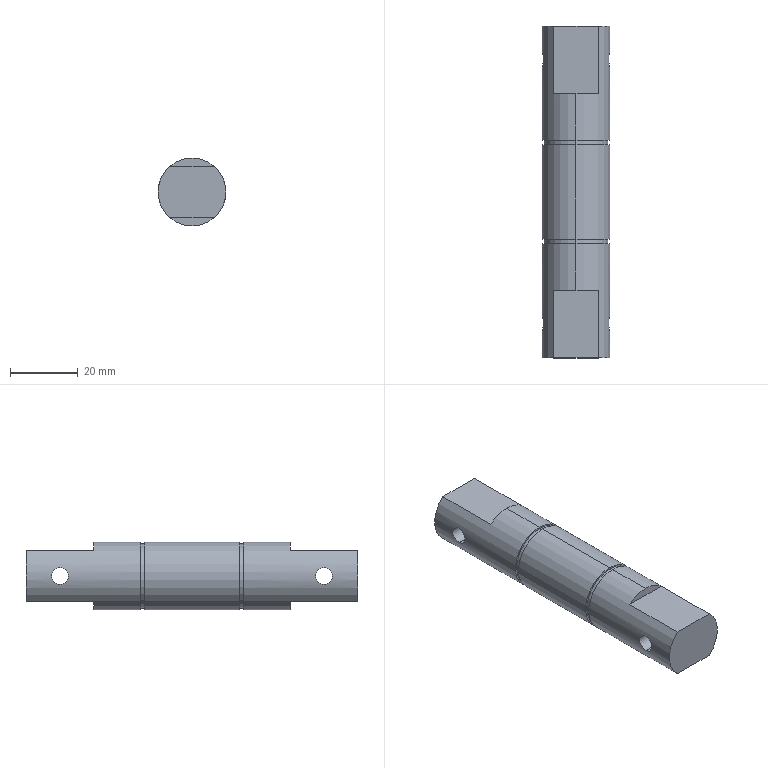Part | SolidWorks | features Extrusion 1, HoleWzd 1, ICE 1, RevCut 1 | 1 solid | 28 faces | box 20 x 98 x 20 mm | volume 28115 mm3 | cylinder 14 | plane 14 | commonest cylinder face diameters 20 x6 5 x4 19 x4
STEP:
#1=CARTESIAN_POINT('',(9.682,10.,-2.5));
#2=VERTEX_POINT('',#1);
#3=CARTESIAN_POINT('',(9.682,10.,2.5));
#4=VERTEX_POINT('',#3);
#5=CARTESIAN_POINT('',(9.682,10.,-2.5));
#6=CARTESIAN_POINT('',(9.682,9.834,-2.5));
#7=CARTESIAN_POINT('',(9.687,9.671,-2.484));
#8=CARTESIAN_POINT('',(9.703,9.351,-2.42));
#9=CARTESIAN_POINT('',(9.715,9.192,-2.371));
#10=CARTESIAN_POINT('',(9.745,8.889,-2.246));
#11=CARTESIAN_POINT('',(9.762,8.746,-2.169));
#12=CARTESIAN_POINT('',(9.801,8.475,-1.987));
#13=CARTESIAN_POINT('',(9.822,8.347,-1.882));
#14=CARTESIAN_POINT('',(9.884,8.002,-1.538));
#15=CARTESIAN_POINT('',(9.925,7.816,-1.26));
#16=CARTESIAN_POINT('',(9.968,7.629,-0.8089));
#17=CARTESIAN_POINT('',(9.98,7.581,-0.6506));
#18=CARTESIAN_POINT('',(9.996,7.516,-0.3275));
#19=CARTESIAN_POINT('',(10.,7.5,-0.1648));
#20=CARTESIAN_POINT('',(10.,7.5,0.1628));
#21=CARTESIAN_POINT('',(9.996,7.516,0.3292));
#22=CARTESIAN_POINT('',(9.98,7.581,0.6504));
#23=CARTESIAN_POINT('',(9.969,7.628,0.8066));
#24=CARTESIAN_POINT('',(9.925,7.817,1.262));
#25=CARTESIAN_POINT('',(9.884,8.001,1.537));
#26=CARTESIAN_POINT('',(9.822,8.349,1.884));
#27=CARTESIAN_POINT('',(9.801,8.474,1.987));
#28=CARTESIAN_POINT('',(9.763,8.744,2.168));
#29=CARTESIAN_POINT('',(9.745,8.891,2.246));
#30=CARTESIAN_POINT('',(9.715,9.193,2.372));
#31=CARTESIAN_POINT('',(9.703,9.348,2.419));
#32=CARTESIAN_POINT('',(9.687,9.67,2.484));
#33=CARTESIAN_POINT('',(9.682,9.836,2.5));
#34=CARTESIAN_POINT('',(9.682,10.,2.5));
#35=B_SPLINE_CURVE_WITH_KNOTS('',3,(#5,#6,#7,#8,#9,#10,#11,#12,#13,#14,#15,#16,#17,#18,#19,#20,#21,#22,#23,#24,#25,#26,#27,#28,#29,#30,#31,#32,#33,#34),.UNSPECIFIED.,.F.,.F.,(4,2,2,2,2,2,2,2,2,2,2,2,2,2,4),(0.,0.0004905,0.0009809,0.001471,0.001962,0.002943,0.003433,0.003924,0.004414,0.004905,0.005885,0.006376,0.006866,0.007357,0.007847),.UNSPECIFIED.);
#36=EDGE_CURVE('',#2,#4,#35,.T.);
#37=ORIENTED_EDGE('',*,*,#36,.T.);
#38=CARTESIAN_POINT('',(9.682,10.,2.5));
#39=CARTESIAN_POINT('',(9.682,10.327,2.5));
#40=CARTESIAN_POINT('',(9.7,10.657,2.434));
#41=CARTESIAN_POINT('',(9.745,11.109,2.247));
#42=CARTESIAN_POINT('',(9.763,11.255,2.168));
#43=CARTESIAN_POINT('',(9.801,11.526,1.987));
#44=CARTESIAN_POINT('',(9.822,11.652,1.884));
#45=CARTESIAN_POINT('',(9.863,11.882,1.653));
#46=CARTESIAN_POINT('',(9.884,11.987,1.526));
#47=CARTESIAN_POINT('',(9.922,12.168,1.255));
#48=CARTESIAN_POINT('',(9.939,12.245,1.112));
#49=CARTESIAN_POINT('',(9.968,12.372,0.808));
#50=CARTESIAN_POINT('',(9.98,12.419,0.6507));
#51=CARTESIAN_POINT('',(9.996,12.483,0.3307));
#52=CARTESIAN_POINT('',(10.,12.5,0.1656));
#53=CARTESIAN_POINT('',(10.,12.5,-0.1641));
#54=CARTESIAN_POINT('',(9.996,12.484,-0.3268));
#55=CARTESIAN_POINT('',(9.98,12.42,-0.6479));
#56=CARTESIAN_POINT('',(9.968,12.372,-0.8075));
#57=CARTESIAN_POINT('',(9.939,12.246,-1.109));
#58=CARTESIAN_POINT('',(9.922,12.17,-1.253));
#59=CARTESIAN_POINT('',(9.884,11.988,-1.525));
#60=CARTESIAN_POINT('',(9.863,11.883,-1.652));
#61=CARTESIAN_POINT('',(9.822,11.654,-1.882));
#62=CARTESIAN_POINT('',(9.801,11.527,-1.986));
#63=CARTESIAN_POINT('',(9.763,11.255,-2.168));
#64=CARTESIAN_POINT('',(9.745,11.112,-2.245));
#65=CARTESIAN_POINT('',(9.715,10.811,-2.371));
#66=CARTESIAN_POINT('',(9.703,10.651,-2.419));
#67=CARTESIAN_POINT('',(9.687,10.329,-2.484));
#68=CARTESIAN_POINT('',(9.682,10.166,-2.5));
#69=CARTESIAN_POINT('',(9.682,10.,-2.5));
#70=B_SPLINE_CURVE_WITH_KNOTS('',3,(#38,#39,#40,#41,#42,#43,#44,#45,#46,#47,#48,#49,#50,#51,#52,#53,#54,#55,#56,#57,#58,#59,#60,#61,#62,#63,#64,#65,#66,#67,#68,#69),.UNSPECIFIED.,.F.,.F.,(4,2,2,2,2,2,2,2,2,2,2,2,2,2,2,4),(0.007847,0.008828,0.009318,0.009809,0.0103,0.01079,0.01128,0.01177,0.01226,0.01275,0.01324,0.01373,0.01422,0.01471,0.0152,0.01569),.UNSPECIFIED.);
#71=EDGE_CURVE('',#4,#2,#70,.T.);
#72=ORIENTED_EDGE('',*,*,#71,.T.);
#73=EDGE_LOOP('',(#37,#72));
#74=FACE_BOUND('',#73,.T.);
#75=CARTESIAN_POINT('',(0.,33.7,10.));
#76=VERTEX_POINT('',#75);
#77=CARTESIAN_POINT('',(0.,33.7,-10.));
#78=VERTEX_POINT('',#77);
#79=CARTESIAN_POINT('',(0.,33.7,0.));
#80=DIRECTION('',(0.,1.,0.));
#81=DIRECTION('',(0.,0.,1.));
#82=AXIS2_PLACEMENT_3D('',#79,#80,#81);
#83=CIRCLE('',#82,10.);
#84=EDGE_CURVE('',#76,#78,#83,.T.);
#85=ORIENTED_EDGE('',*,*,#84,.F.);
#86=CARTESIAN_POINT('',(0.,20.,10.));
#87=VERTEX_POINT('',#86);
#88=CARTESIAN_POINT('',(0.,98.,10.));
#89=DIRECTION('',(0.,-1.,0.));
#90=VECTOR('',#89,1000.);
#91=LINE('',#88,#90);
#92=EDGE_CURVE('',#76,#87,#91,.T.);
#93=ORIENTED_EDGE('',*,*,#92,.T.);
#94=CARTESIAN_POINT('',(6.614,20.,7.5));
#95=VERTEX_POINT('',#94);
#96=CARTESIAN_POINT('',(0.,20.,0.));
#97=DIRECTION('',(0.,-1.,0.));
#98=DIRECTION('',(0.,0.,-1.));
#99=AXIS2_PLACEMENT_3D('',#96,#97,#98);
#100=CIRCLE('',#99,10.);
#101=EDGE_CURVE('',#95,#87,#100,.T.);
#102=ORIENTED_EDGE('',*,*,#101,.F.);
#103=CARTESIAN_POINT('',(6.614,0.,7.5));
#104=VERTEX_POINT('',#103);
#105=CARTESIAN_POINT('',(6.614,98.,7.5));
#106=DIRECTION('',(0.,1.,0.));
#107=VECTOR('',#106,1000.);
#108=LINE('',#105,#107);
#109=EDGE_CURVE('',#104,#95,#108,.T.);
#110=ORIENTED_EDGE('',*,*,#109,.F.);
#111=CARTESIAN_POINT('',(6.614,0.,-7.5));
#112=VERTEX_POINT('',#111);
#113=CARTESIAN_POINT('',(0.,0.,0.));
#114=DIRECTION('',(0.,1.,0.));
#115=DIRECTION('',(0.,0.,1.));
#116=AXIS2_PLACEMENT_3D('',#113,#114,#115);
#117=CIRCLE('',#116,10.);
#118=EDGE_CURVE('',#104,#112,#117,.T.);
#119=ORIENTED_EDGE('',*,*,#118,.T.);
#120=CARTESIAN_POINT('',(6.614,20.,-7.5));
#121=VERTEX_POINT('',#120);
#122=CARTESIAN_POINT('',(6.614,98.,-7.5));
#123=DIRECTION('',(0.,-1.,0.));
#124=VECTOR('',#123,1000.);
#125=LINE('',#122,#124);
#126=EDGE_CURVE('',#121,#112,#125,.T.);
#127=ORIENTED_EDGE('',*,*,#126,.F.);
#128=CARTESIAN_POINT('',(0.,20.,-10.));
#129=VERTEX_POINT('',#128);
#130=CARTESIAN_POINT('',(0.,20.,0.));
#131=DIRECTION('',(0.,-1.,0.));
#132=DIRECTION('',(0.,0.,-1.));
#133=AXIS2_PLACEMENT_3D('',#130,#131,#132);
#134=CIRCLE('',#133,10.);
#135=EDGE_CURVE('',#129,#121,#134,.T.);
#136=ORIENTED_EDGE('',*,*,#135,.F.);
#137=CARTESIAN_POINT('',(0.,98.,-10.));
#138=DIRECTION('',(0.,-1.,0.));
#139=VECTOR('',#138,1000.);
#140=LINE('',#137,#139);
#141=EDGE_CURVE('',#78,#129,#140,.T.);
#142=ORIENTED_EDGE('',*,*,#141,.F.);
#143=EDGE_LOOP('',(#85,#93,#102,#110,#119,#127,#136,#142));
#144=FACE_OUTER_BOUND('',#143,.T.);
#145=CARTESIAN_POINT('',(0.,98.,0.));
#146=DIRECTION('',(0.,-1.,0.));
#147=DIRECTION('',(0.,0.,-1.));
#148=AXIS2_PLACEMENT_3D('',#145,#146,#147);
#149=CYLINDRICAL_SURFACE('',#148,10.);
#150=ADVANCED_FACE('',(#74,#144),#149,.T.);
#151=CARTESIAN_POINT('',(-9.682,10.,2.5));
#152=VERTEX_POINT('',#151);
#153=CARTESIAN_POINT('',(-9.682,10.,-2.5));
#154=VERTEX_POINT('',#153);
#155=CARTESIAN_POINT('',(-9.682,10.,2.5));
#156=CARTESIAN_POINT('',(-9.682,9.835,2.5));
#157=CARTESIAN_POINT('',(-9.687,9.672,2.484));
#158=CARTESIAN_POINT('',(-9.703,9.351,2.42));
#159=CARTESIAN_POINT('',(-9.715,9.192,2.371));
#160=CARTESIAN_POINT('',(-9.745,8.89,2.246));
#161=CARTESIAN_POINT('',(-9.762,8.747,2.169));
#162=CARTESIAN_POINT('',(-9.801,8.474,1.987));
#163=CARTESIAN_POINT('',(-9.822,8.347,1.883));
#164=CARTESIAN_POINT('',(-9.863,8.118,1.653));
#165=CARTESIAN_POINT('',(-9.884,8.013,1.526));
#166=CARTESIAN_POINT('',(-9.922,7.831,1.254));
#167=CARTESIAN_POINT('',(-9.939,7.754,1.111));
#168=CARTESIAN_POINT('',(-9.968,7.629,0.8095));
#169=CARTESIAN_POINT('',(-9.98,7.58,0.6502));
#170=CARTESIAN_POINT('',(-9.996,7.516,0.3279));
#171=CARTESIAN_POINT('',(-10.,7.5,0.1644));
#172=CARTESIAN_POINT('',(-10.,7.5,-0.1673));
#173=CARTESIAN_POINT('',(-9.996,7.517,-0.3303));
#174=CARTESIAN_POINT('',(-9.98,7.581,-0.6507));
#175=CARTESIAN_POINT('',(-9.968,7.629,-0.8098));
#176=CARTESIAN_POINT('',(-9.939,7.755,-1.112));
#177=CARTESIAN_POINT('',(-9.922,7.832,-1.255));
#178=CARTESIAN_POINT('',(-9.884,8.014,-1.527));
#179=CARTESIAN_POINT('',(-9.863,8.119,-1.654));
#180=CARTESIAN_POINT('',(-9.801,8.463,-1.999));
#181=CARTESIAN_POINT('',(-9.759,8.741,-2.184));
#182=CARTESIAN_POINT('',(-9.715,9.192,-2.371));
#183=CARTESIAN_POINT('',(-9.703,9.351,-2.42));
#184=CARTESIAN_POINT('',(-9.687,9.674,-2.484));
#185=CARTESIAN_POINT('',(-9.682,9.836,-2.5));
#186=CARTESIAN_POINT('',(-9.682,10.,-2.5));
#187=B_SPLINE_CURVE_WITH_KNOTS('',3,(#155,#156,#157,#158,#159,#160,#161,#162,#163,#164,#165,#166,#167,#168,#169,#170,#171,#172,#173,#174,#175,#176,#177,#178,#179,#180,#181,#182,#183,#184,#185,#186),.UNSPECIFIED.,.F.,.F.,(4,2,2,2,2,2,2,2,2,2,2,2,2,2,2,4),(0.01177,0.01226,0.01275,0.01324,0.01373,0.01422,0.01471,0.0152,0.01569,0.01618,0.01667,0.01717,0.01766,0.01864,0.01913,0.01962),.UNSPECIFIED.);
#188=EDGE_CURVE('',#152,#154,#187,.T.);
#189=ORIENTED_EDGE('',*,*,#188,.F.);
#190=CARTESIAN_POINT('',(10.,10.,2.5));
#191=DIRECTION('',(1.,0.,0.));
#192=VECTOR('',#191,1000.);
#193=LINE('',#190,#192);
#194=EDGE_CURVE('',#152,#4,#193,.T.);
#195=ORIENTED_EDGE('',*,*,#194,.T.);
#196=ORIENTED_EDGE('',*,*,#36,.F.);
#197=CARTESIAN_POINT('',(10.,10.,-2.5));
#198=DIRECTION('',(1.,0.,0.));
#199=VECTOR('',#198,1000.);
#200=LINE('',#197,#199);
#201=EDGE_CURVE('',#154,#2,#200,.T.);
#202=ORIENTED_EDGE('',*,*,#201,.F.);
#203=EDGE_LOOP('',(#189,#195,#196,#202));
#204=FACE_OUTER_BOUND('',#203,.T.);
#205=CARTESIAN_POINT('',(10.,10.,0.));
#206=DIRECTION('',(1.,0.,0.));
#207=DIRECTION('',(0.,0.,-1.));
#208=AXIS2_PLACEMENT_3D('',#205,#206,#207);
#209=CYLINDRICAL_SURFACE('',#208,2.5);
#210=ADVANCED_FACE('',(#204),#209,.F.);
#211=CARTESIAN_POINT('',(0.,33.7,9.5));
#212=VERTEX_POINT('',#211);
#213=CARTESIAN_POINT('',(0.,33.7,-9.5));
#214=VERTEX_POINT('',#213);
#215=CARTESIAN_POINT('',(0.,33.7,0.));
#216=DIRECTION('',(0.,1.,0.));
#217=DIRECTION('',(0.,0.,1.));
#218=AXIS2_PLACEMENT_3D('',#215,#216,#217);
#219=CIRCLE('',#218,9.5);
#220=EDGE_CURVE('',#212,#214,#219,.T.);
#221=ORIENTED_EDGE('',*,*,#220,.T.);
#222=CARTESIAN_POINT('',(0.,35.,-9.5));
#223=VERTEX_POINT('',#222);
#224=CARTESIAN_POINT('',(0.,98.,-9.5));
#225=DIRECTION('',(0.,1.,0.));
#226=VECTOR('',#225,1000.);
#227=LINE('',#224,#226);
#228=EDGE_CURVE('',#214,#223,#227,.T.);
#229=ORIENTED_EDGE('',*,*,#228,.T.);
#230=CARTESIAN_POINT('',(0.,35.,9.5));
#231=VERTEX_POINT('',#230);
#232=CARTESIAN_POINT('',(0.,35.,0.));
#233=DIRECTION('',(0.,1.,0.));
#234=DIRECTION('',(0.,0.,1.));
#235=AXIS2_PLACEMENT_3D('',#232,#233,#234);
#236=CIRCLE('',#235,9.5);
#237=EDGE_CURVE('',#231,#223,#236,.T.);
#238=ORIENTED_EDGE('',*,*,#237,.F.);
#239=CARTESIAN_POINT('',(0.,98.,9.5));
#240=DIRECTION('',(0.,1.,0.));
#241=VECTOR('',#240,1000.);
#242=LINE('',#239,#241);
#243=EDGE_CURVE('',#212,#231,#242,.T.);
#244=ORIENTED_EDGE('',*,*,#243,.F.);
#245=EDGE_LOOP('',(#221,#229,#238,#244));
#246=FACE_OUTER_BOUND('',#245,.T.);
#247=CARTESIAN_POINT('',(0.,98.,0.));
#248=DIRECTION('',(0.,1.,0.));
#249=DIRECTION('',(0.,0.,1.));
#250=AXIS2_PLACEMENT_3D('',#247,#248,#249);
#251=CYLINDRICAL_SURFACE('',#250,9.5);
#252=ADVANCED_FACE('',(#246),#251,.T.);
#253=CARTESIAN_POINT('',(0.,63.,10.));
#254=VERTEX_POINT('',#253);
#255=CARTESIAN_POINT('',(0.,63.,-10.));
#256=VERTEX_POINT('',#255);
#257=CARTESIAN_POINT('',(0.,63.,0.));
#258=DIRECTION('',(0.,1.,0.));
#259=DIRECTION('',(0.,0.,1.));
#260=AXIS2_PLACEMENT_3D('',#257,#258,#259);
#261=CIRCLE('',#260,10.);
#262=EDGE_CURVE('',#254,#256,#261,.T.);
#263=ORIENTED_EDGE('',*,*,#262,.F.);
#264=CARTESIAN_POINT('',(0.,35.,10.));
#265=VERTEX_POINT('',#264);
#266=CARTESIAN_POINT('',(0.,98.,10.));
#267=DIRECTION('',(0.,-1.,0.));
#268=VECTOR('',#267,1000.);
#269=LINE('',#266,#268);
#270=EDGE_CURVE('',#254,#265,#269,.T.);
#271=ORIENTED_EDGE('',*,*,#270,.T.);
#272=CARTESIAN_POINT('',(0.,35.,-10.));
#273=VERTEX_POINT('',#272);
#274=CARTESIAN_POINT('',(0.,35.,0.));
#275=DIRECTION('',(0.,1.,0.));
#276=DIRECTION('',(0.,0.,1.));
#277=AXIS2_PLACEMENT_3D('',#274,#275,#276);
#278=CIRCLE('',#277,10.);
#279=EDGE_CURVE('',#265,#273,#278,.T.);
#280=ORIENTED_EDGE('',*,*,#279,.T.);
#281=CARTESIAN_POINT('',(0.,98.,-10.));
#282=DIRECTION('',(0.,-1.,0.));
#283=VECTOR('',#282,1000.);
#284=LINE('',#281,#283);
#285=EDGE_CURVE('',#256,#273,#284,.T.);
#286=ORIENTED_EDGE('',*,*,#285,.F.);
#287=EDGE_LOOP('',(#263,#271,#280,#286));
#288=FACE_OUTER_BOUND('',#287,.T.);
#289=CARTESIAN_POINT('',(0.,98.,0.));
#290=DIRECTION('',(0.,-1.,0.));
#291=DIRECTION('',(0.,0.,-1.));
#292=AXIS2_PLACEMENT_3D('',#289,#290,#291);
#293=CYLINDRICAL_SURFACE('',#292,10.);
#294=ADVANCED_FACE('',(#288),#293,.T.);
#295=CARTESIAN_POINT('',(0.,63.,9.5));
#296=VERTEX_POINT('',#295);
#297=CARTESIAN_POINT('',(0.,63.,-9.5));
#298=VERTEX_POINT('',#297);
#299=CARTESIAN_POINT('',(0.,63.,0.));
#300=DIRECTION('',(0.,1.,0.));
#301=DIRECTION('',(0.,0.,1.));
#302=AXIS2_PLACEMENT_3D('',#299,#300,#301);
#303=CIRCLE('',#302,9.5);
#304=EDGE_CURVE('',#296,#298,#303,.T.);
#305=ORIENTED_EDGE('',*,*,#304,.T.);
#306=CARTESIAN_POINT('',(0.,64.3,-9.5));
#307=VERTEX_POINT('',#306);
#308=CARTESIAN_POINT('',(0.,98.,-9.5));
#309=DIRECTION('',(0.,1.,0.));
#310=VECTOR('',#309,1000.);
#311=LINE('',#308,#310);
#312=EDGE_CURVE('',#298,#307,#311,.T.);
#313=ORIENTED_EDGE('',*,*,#312,.T.);
#314=CARTESIAN_POINT('',(0.,64.3,9.5));
#315=VERTEX_POINT('',#314);
#316=CARTESIAN_POINT('',(0.,64.3,0.));
#317=DIRECTION('',(0.,1.,0.));
#318=DIRECTION('',(0.,0.,1.));
#319=AXIS2_PLACEMENT_3D('',#316,#317,#318);
#320=CIRCLE('',#319,9.5);
#321=EDGE_CURVE('',#315,#307,#320,.T.);
#322=ORIENTED_EDGE('',*,*,#321,.F.);
#323=CARTESIAN_POINT('',(0.,98.,9.5));
#324=DIRECTION('',(0.,1.,0.));
#325=VECTOR('',#324,1000.);
#326=LINE('',#323,#325);
#327=EDGE_CURVE('',#296,#315,#326,.T.);
#328=ORIENTED_EDGE('',*,*,#327,.F.);
#329=EDGE_LOOP('',(#305,#313,#322,#328));
#330=FACE_OUTER_BOUND('',#329,.T.);
#331=CARTESIAN_POINT('',(0.,98.,0.));
#332=DIRECTION('',(0.,1.,0.));
#333=DIRECTION('',(0.,0.,1.));
#334=AXIS2_PLACEMENT_3D('',#331,#332,#333);
#335=CYLINDRICAL_SURFACE('',#334,9.5);
#336=ADVANCED_FACE('',(#330),#335,.T.);
#337=CARTESIAN_POINT('',(-9.682,88.,2.5));
#338=VERTEX_POINT('',#337);
#339=CARTESIAN_POINT('',(-9.682,88.,-2.5));
#340=VERTEX_POINT('',#339);
#341=CARTESIAN_POINT('',(-9.682,88.,2.5));
#342=CARTESIAN_POINT('',(-9.682,87.835,2.5));
#343=CARTESIAN_POINT('',(-9.687,87.672,2.484));
#344=CARTESIAN_POINT('',(-9.703,87.351,2.42));
#345=CARTESIAN_POINT('',(-9.715,87.192,2.371));
#346=CARTESIAN_POINT('',(-9.745,86.89,2.246));
#347=CARTESIAN_POINT('',(-9.762,86.747,2.169));
#348=CARTESIAN_POINT('',(-9.801,86.474,1.987));
#349=CARTESIAN_POINT('',(-9.822,86.347,1.883));
#350=CARTESIAN_POINT('',(-9.863,86.118,1.653));
#351=CARTESIAN_POINT('',(-9.884,86.013,1.526));
#352=CARTESIAN_POINT('',(-9.922,85.831,1.254));
#353=CARTESIAN_POINT('',(-9.939,85.754,1.111));
#354=CARTESIAN_POINT('',(-9.968,85.629,0.8095));
#355=CARTESIAN_POINT('',(-9.98,85.58,0.6502));
#356=CARTESIAN_POINT('',(-9.996,85.516,0.3279));
#357=CARTESIAN_POINT('',(-10.,85.5,0.1644));
#358=CARTESIAN_POINT('',(-10.,85.5,-0.1673));
#359=CARTESIAN_POINT('',(-9.996,85.517,-0.3303));
#360=CARTESIAN_POINT('',(-9.98,85.581,-0.6507));
#361=CARTESIAN_POINT('',(-9.968,85.629,-0.8098));
#362=CARTESIAN_POINT('',(-9.939,85.755,-1.112));
#363=CARTESIAN_POINT('',(-9.922,85.832,-1.255));
#364=CARTESIAN_POINT('',(-9.884,86.014,-1.527));
#365=CARTESIAN_POINT('',(-9.863,86.119,-1.654));
#366=CARTESIAN_POINT('',(-9.801,86.463,-1.999));
#367=CARTESIAN_POINT('',(-9.759,86.741,-2.184));
#368=CARTESIAN_POINT('',(-9.715,87.192,-2.371));
#369=CARTESIAN_POINT('',(-9.703,87.351,-2.42));
#370=CARTESIAN_POINT('',(-9.687,87.674,-2.484));
#371=CARTESIAN_POINT('',(-9.682,87.836,-2.5));
#372=CARTESIAN_POINT('',(-9.682,88.,-2.5));
#373=B_SPLINE_CURVE_WITH_KNOTS('',3,(#341,#342,#343,#344,#345,#346,#347,#348,#349,#350,#351,#352,#353,#354,#355,#356,#357,#358,#359,#360,#361,#362,#363,#364,#365,#366,#367,#368,#369,#370,#371,#372),.UNSPECIFIED.,.F.,.F.,(4,2,2,2,2,2,2,2,2,2,2,2,2,2,2,4),(0.01177,0.01226,0.01275,0.01324,0.01373,0.01422,0.01471,0.0152,0.01569,0.01618,0.01667,0.01717,0.01766,0.01864,0.01913,0.01962),.UNSPECIFIED.);
#374=EDGE_CURVE('',#338,#340,#373,.T.);
#375=ORIENTED_EDGE('',*,*,#374,.F.);
#376=CARTESIAN_POINT('',(9.682,88.,2.5));
#377=VERTEX_POINT('',#376);
#378=CARTESIAN_POINT('',(10.,88.,2.5));
#379=DIRECTION('',(1.,0.,0.));
#380=VECTOR('',#379,1000.);
#381=LINE('',#378,#380);
#382=EDGE_CURVE('',#338,#377,#381,.T.);
#383=ORIENTED_EDGE('',*,*,#382,.T.);
#384=CARTESIAN_POINT('',(9.682,88.,-2.5));
#385=VERTEX_POINT('',#384);
#386=CARTESIAN_POINT('',(9.682,88.,-2.5));
#387=CARTESIAN_POINT('',(9.682,87.834,-2.5));
#388=CARTESIAN_POINT('',(9.687,87.671,-2.484));
#389=CARTESIAN_POINT('',(9.703,87.351,-2.42));
#390=CARTESIAN_POINT('',(9.715,87.192,-2.371));
#391=CARTESIAN_POINT('',(9.745,86.889,-2.246));
#392=CARTESIAN_POINT('',(9.762,86.746,-2.169));
#393=CARTESIAN_POINT('',(9.801,86.475,-1.987));
#394=CARTESIAN_POINT('',(9.822,86.347,-1.882));
#395=CARTESIAN_POINT('',(9.884,86.002,-1.538));
#396=CARTESIAN_POINT('',(9.925,85.816,-1.26));
#397=CARTESIAN_POINT('',(9.968,85.629,-0.8089));
#398=CARTESIAN_POINT('',(9.98,85.581,-0.6506));
#399=CARTESIAN_POINT('',(9.996,85.516,-0.3275));
#400=CARTESIAN_POINT('',(10.,85.5,-0.1648));
#401=CARTESIAN_POINT('',(10.,85.5,0.1628));
#402=CARTESIAN_POINT('',(9.996,85.516,0.3292));
#403=CARTESIAN_POINT('',(9.98,85.581,0.6504));
#404=CARTESIAN_POINT('',(9.969,85.628,0.8066));
#405=CARTESIAN_POINT('',(9.925,85.817,1.262));
#406=CARTESIAN_POINT('',(9.884,86.001,1.537));
#407=CARTESIAN_POINT('',(9.822,86.349,1.884));
#408=CARTESIAN_POINT('',(9.801,86.474,1.987));
#409=CARTESIAN_POINT('',(9.763,86.744,2.168));
#410=CARTESIAN_POINT('',(9.745,86.891,2.246));
#411=CARTESIAN_POINT('',(9.715,87.193,2.372));
#412=CARTESIAN_POINT('',(9.703,87.348,2.419));
#413=CARTESIAN_POINT('',(9.687,87.67,2.484));
#414=CARTESIAN_POINT('',(9.682,87.836,2.5));
#415=CARTESIAN_POINT('',(9.682,88.,2.5));
#416=B_SPLINE_CURVE_WITH_KNOTS('',3,(#386,#387,#388,#389,#390,#391,#392,#393,#394,#395,#396,#397,#398,#399,#400,#401,#402,#403,#404,#405,#406,#407,#408,#409,#410,#411,#412,#413,#414,#415),.UNSPECIFIED.,.F.,.F.,(4,2,2,2,2,2,2,2,2,2,2,2,2,2,4),(0.,0.0004905,0.0009809,0.001471,0.001962,0.002943,0.003433,0.003924,0.004414,0.004905,0.005885,0.006376,0.006866,0.007357,0.007847),.UNSPECIFIED.);
#417=EDGE_CURVE('',#385,#377,#416,.T.);
#418=ORIENTED_EDGE('',*,*,#417,.F.);
#419=CARTESIAN_POINT('',(10.,88.,-2.5));
#420=DIRECTION('',(1.,0.,0.));
#421=VECTOR('',#420,1000.);
#422=LINE('',#419,#421);
#423=EDGE_CURVE('',#340,#385,#422,.T.);
#424=ORIENTED_EDGE('',*,*,#423,.F.);
#425=EDGE_LOOP('',(#375,#383,#418,#424));
#426=FACE_OUTER_BOUND('',#425,.T.);
#427=CARTESIAN_POINT('',(10.,88.,0.));
#428=DIRECTION('',(1.,0.,0.));
#429=DIRECTION('',(0.,0.,-1.));
#430=AXIS2_PLACEMENT_3D('',#427,#428,#429);
#431=CYLINDRICAL_SURFACE('',#430,2.5);
#432=ADVANCED_FACE('',(#426),#431,.F.);
#433=ORIENTED_EDGE('',*,*,#417,.T.);
#434=CARTESIAN_POINT('',(9.682,88.,2.5));
#435=CARTESIAN_POINT('',(9.682,88.327,2.5));
#436=CARTESIAN_POINT('',(9.7,88.657,2.434));
#437=CARTESIAN_POINT('',(9.745,89.109,2.247));
#438=CARTESIAN_POINT('',(9.763,89.255,2.168));
#439=CARTESIAN_POINT('',(9.801,89.526,1.987));
#440=CARTESIAN_POINT('',(9.822,89.652,1.884));
#441=CARTESIAN_POINT('',(9.863,89.882,1.653));
#442=CARTESIAN_POINT('',(9.884,89.987,1.526));
#443=CARTESIAN_POINT('',(9.922,90.168,1.255));
#444=CARTESIAN_POINT('',(9.939,90.245,1.112));
#445=CARTESIAN_POINT('',(9.968,90.372,0.808));
#446=CARTESIAN_POINT('',(9.98,90.419,0.6507));
#447=CARTESIAN_POINT('',(9.996,90.483,0.3307));
#448=CARTESIAN_POINT('',(10.,90.5,0.1656));
#449=CARTESIAN_POINT('',(10.,90.5,-0.1641));
#450=CARTESIAN_POINT('',(9.996,90.484,-0.3268));
#451=CARTESIAN_POINT('',(9.98,90.42,-0.6479));
#452=CARTESIAN_POINT('',(9.968,90.372,-0.8075));
#453=CARTESIAN_POINT('',(9.939,90.246,-1.109));
#454=CARTESIAN_POINT('',(9.922,90.17,-1.253));
#455=CARTESIAN_POINT('',(9.884,89.988,-1.525));
#456=CARTESIAN_POINT('',(9.863,89.883,-1.652));
#457=CARTESIAN_POINT('',(9.822,89.654,-1.882));
#458=CARTESIAN_POINT('',(9.801,89.527,-1.986));
#459=CARTESIAN_POINT('',(9.763,89.255,-2.168));
#460=CARTESIAN_POINT('',(9.745,89.112,-2.245));
#461=CARTESIAN_POINT('',(9.715,88.811,-2.371));
#462=CARTESIAN_POINT('',(9.703,88.651,-2.419));
#463=CARTESIAN_POINT('',(9.687,88.329,-2.484));
#464=CARTESIAN_POINT('',(9.682,88.166,-2.5));
#465=CARTESIAN_POINT('',(9.682,88.,-2.5));
#466=B_SPLINE_CURVE_WITH_KNOTS('',3,(#434,#435,#436,#437,#438,#439,#440,#441,#442,#443,#444,#445,#446,#447,#448,#449,#450,#451,#452,#453,#454,#455,#456,#457,#458,#459,#460,#461,#462,#463,#464,#465),.UNSPECIFIED.,.F.,.F.,(4,2,2,2,2,2,2,2,2,2,2,2,2,2,2,4),(0.007847,0.008828,0.009318,0.009809,0.0103,0.01079,0.01128,0.01177,0.01226,0.01275,0.01324,0.01373,0.01422,0.01471,0.0152,0.01569),.UNSPECIFIED.);
#467=EDGE_CURVE('',#377,#385,#466,.T.);
#468=ORIENTED_EDGE('',*,*,#467,.T.);
#469=EDGE_LOOP('',(#433,#468));
#470=FACE_BOUND('',#469,.T.);
#471=CARTESIAN_POINT('',(0.,78.,10.));
#472=VERTEX_POINT('',#471);
#473=CARTESIAN_POINT('',(6.614,78.,7.5));
#474=VERTEX_POINT('',#473);
#475=CARTESIAN_POINT('',(0.,78.,0.));
#476=DIRECTION('',(0.,1.,0.));
#477=DIRECTION('',(0.,0.,1.));
#478=AXIS2_PLACEMENT_3D('',#475,#476,#477);
#479=CIRCLE('',#478,10.);
#480=EDGE_CURVE('',#472,#474,#479,.T.);
#481=ORIENTED_EDGE('',*,*,#480,.F.);
#482=CARTESIAN_POINT('',(0.,64.3,10.));
#483=VERTEX_POINT('',#482);
#484=CARTESIAN_POINT('',(0.,98.,10.));
#485=DIRECTION('',(0.,-1.,0.));
#486=VECTOR('',#485,1000.);
#487=LINE('',#484,#486);
#488=EDGE_CURVE('',#472,#483,#487,.T.);
#489=ORIENTED_EDGE('',*,*,#488,.T.);
#490=CARTESIAN_POINT('',(0.,64.3,-10.));
#491=VERTEX_POINT('',#490);
#492=CARTESIAN_POINT('',(0.,64.3,0.));
#493=DIRECTION('',(0.,1.,0.));
#494=DIRECTION('',(0.,0.,1.));
#495=AXIS2_PLACEMENT_3D('',#492,#493,#494);
#496=CIRCLE('',#495,10.);
#497=EDGE_CURVE('',#483,#491,#496,.T.);
#498=ORIENTED_EDGE('',*,*,#497,.T.);
#499=CARTESIAN_POINT('',(0.,78.,-10.));
#500=VERTEX_POINT('',#499);
#501=CARTESIAN_POINT('',(0.,98.,-10.));
#502=DIRECTION('',(0.,-1.,0.));
#503=VECTOR('',#502,1000.);
#504=LINE('',#501,#503);
#505=EDGE_CURVE('',#500,#491,#504,.T.);
#506=ORIENTED_EDGE('',*,*,#505,.F.);
#507=CARTESIAN_POINT('',(6.614,78.,-7.5));
#508=VERTEX_POINT('',#507);
#509=CARTESIAN_POINT('',(0.,78.,0.));
#510=DIRECTION('',(0.,1.,0.));
#511=DIRECTION('',(0.,0.,1.));
#512=AXIS2_PLACEMENT_3D('',#509,#510,#511);
#513=CIRCLE('',#512,10.);
#514=EDGE_CURVE('',#508,#500,#513,.T.);
#515=ORIENTED_EDGE('',*,*,#514,.F.);
#516=CARTESIAN_POINT('',(6.614,98.,-7.5));
#517=VERTEX_POINT('',#516);
#518=CARTESIAN_POINT('',(6.614,98.,-7.5));
#519=DIRECTION('',(0.,-1.,0.));
#520=VECTOR('',#519,1000.);
#521=LINE('',#518,#520);
#522=EDGE_CURVE('',#517,#508,#521,.T.);
#523=ORIENTED_EDGE('',*,*,#522,.F.);
#524=CARTESIAN_POINT('',(6.614,98.,7.5));
#525=VERTEX_POINT('',#524);
#526=CARTESIAN_POINT('',(0.,98.,0.));
#527=DIRECTION('',(0.,1.,0.));
#528=DIRECTION('',(0.,0.,1.));
#529=AXIS2_PLACEMENT_3D('',#526,#527,#528);
#530=CIRCLE('',#529,10.);
#531=EDGE_CURVE('',#525,#517,#530,.T.);
#532=ORIENTED_EDGE('',*,*,#531,.F.);
#533=CARTESIAN_POINT('',(6.614,98.,7.5));
#534=DIRECTION('',(0.,1.,0.));
#535=VECTOR('',#534,1000.);
#536=LINE('',#533,#535);
#537=EDGE_CURVE('',#474,#525,#536,.T.);
#538=ORIENTED_EDGE('',*,*,#537,.F.);
#539=EDGE_LOOP('',(#481,#489,#498,#506,#515,#523,#532,#538));
#540=FACE_OUTER_BOUND('',#539,.T.);
#541=CARTESIAN_POINT('',(0.,98.,0.));
#542=DIRECTION('',(0.,-1.,0.));
#543=DIRECTION('',(0.,0.,-1.));
#544=AXIS2_PLACEMENT_3D('',#541,#542,#543);
#545=CYLINDRICAL_SURFACE('',#544,10.);
#546=ADVANCED_FACE('',(#470,#540),#545,.T.);
#547=ORIENTED_EDGE('',*,*,#488,.F.);
#548=CARTESIAN_POINT('',(-6.614,78.,7.5));
#549=VERTEX_POINT('',#548);
#550=CARTESIAN_POINT('',(0.,78.,0.));
#551=DIRECTION('',(0.,1.,0.));
#552=DIRECTION('',(0.,0.,1.));
#553=AXIS2_PLACEMENT_3D('',#550,#551,#552);
#554=CIRCLE('',#553,10.);
#555=EDGE_CURVE('',#549,#472,#554,.T.);
#556=ORIENTED_EDGE('',*,*,#555,.F.);
#557=CARTESIAN_POINT('',(-6.614,98.,7.5));
#558=VERTEX_POINT('',#557);
#559=CARTESIAN_POINT('',(-6.614,98.,7.5));
#560=DIRECTION('',(0.,-1.,0.));
#561=VECTOR('',#560,1000.);
#562=LINE('',#559,#561);
#563=EDGE_CURVE('',#558,#549,#562,.T.);
#564=ORIENTED_EDGE('',*,*,#563,.F.);
#565=CARTESIAN_POINT('',(-6.614,98.,-7.5));
#566=VERTEX_POINT('',#565);
#567=CARTESIAN_POINT('',(0.,98.,0.));
#568=DIRECTION('',(0.,1.,0.));
#569=DIRECTION('',(0.,0.,1.));
#570=AXIS2_PLACEMENT_3D('',#567,#568,#569);
#571=CIRCLE('',#570,10.);
#572=EDGE_CURVE('',#566,#558,#571,.T.);
#573=ORIENTED_EDGE('',*,*,#572,.F.);
#574=CARTESIAN_POINT('',(-6.614,78.,-7.5));
#575=VERTEX_POINT('',#574);
#576=CARTESIAN_POINT('',(-6.614,98.,-7.5));
#577=DIRECTION('',(0.,1.,0.));
#578=VECTOR('',#577,1000.);
#579=LINE('',#576,#578);
#580=EDGE_CURVE('',#575,#566,#579,.T.);
#581=ORIENTED_EDGE('',*,*,#580,.F.);
#582=CARTESIAN_POINT('',(0.,78.,0.));
#583=DIRECTION('',(0.,1.,0.));
#584=DIRECTION('',(0.,0.,1.));
#585=AXIS2_PLACEMENT_3D('',#582,#583,#584);
#586=CIRCLE('',#585,10.);
#587=EDGE_CURVE('',#500,#575,#586,.T.);
#588=ORIENTED_EDGE('',*,*,#587,.F.);
#589=ORIENTED_EDGE('',*,*,#505,.T.);
#590=CARTESIAN_POINT('',(0.,64.3,0.));
#591=DIRECTION('',(0.,1.,0.));
#592=DIRECTION('',(0.,0.,1.));
#593=AXIS2_PLACEMENT_3D('',#590,#591,#592);
#594=CIRCLE('',#593,10.);
#595=EDGE_CURVE('',#491,#483,#594,.T.);
#596=ORIENTED_EDGE('',*,*,#595,.T.);
#597=EDGE_LOOP('',(#547,#556,#564,#573,#581,#588,#589,#596));
#598=FACE_OUTER_BOUND('',#597,.T.);
#599=CARTESIAN_POINT('',(-9.682,88.,-2.5));
#600=CARTESIAN_POINT('',(-9.682,88.164,-2.5));
#601=CARTESIAN_POINT('',(-9.687,88.33,-2.484));
#602=CARTESIAN_POINT('',(-9.703,88.651,-2.419));
#603=CARTESIAN_POINT('',(-9.715,88.807,-2.372));
#604=CARTESIAN_POINT('',(-9.76,89.263,-2.183));
#605=CARTESIAN_POINT('',(-9.801,89.537,-1.999));
#606=CARTESIAN_POINT('',(-9.863,89.884,-1.651));
#607=CARTESIAN_POINT('',(-9.884,89.987,-1.526));
#608=CARTESIAN_POINT('',(-9.922,90.168,-1.255));
#609=CARTESIAN_POINT('',(-9.94,90.247,-1.109));
#610=CARTESIAN_POINT('',(-9.969,90.372,-0.807));
#611=CARTESIAN_POINT('',(-9.98,90.419,-0.6511));
#612=CARTESIAN_POINT('',(-9.996,90.484,-0.3291));
#613=CARTESIAN_POINT('',(-10.,90.5,-0.1631));
#614=CARTESIAN_POINT('',(-10.,90.5,0.3274));
#615=CARTESIAN_POINT('',(-9.983,90.434,0.6576));
#616=CARTESIAN_POINT('',(-9.939,90.246,1.109));
#617=CARTESIAN_POINT('',(-9.922,90.168,1.256));
#618=CARTESIAN_POINT('',(-9.884,89.986,1.527));
#619=CARTESIAN_POINT('',(-9.863,89.883,1.652));
#620=CARTESIAN_POINT('',(-9.822,89.653,1.883));
#621=CARTESIAN_POINT('',(-9.801,89.525,1.988));
#622=CARTESIAN_POINT('',(-9.763,89.255,2.168));
#623=CARTESIAN_POINT('',(-9.745,89.111,2.245));
#624=CARTESIAN_POINT('',(-9.715,88.807,2.372));
#625=CARTESIAN_POINT('',(-9.703,88.65,2.42));
#626=CARTESIAN_POINT('',(-9.687,88.33,2.483));
#627=CARTESIAN_POINT('',(-9.682,88.165,2.5));
#628=CARTESIAN_POINT('',(-9.682,88.,2.5));
#629=B_SPLINE_CURVE_WITH_KNOTS('',3,(#599,#600,#601,#602,#603,#604,#605,#606,#607,#608,#609,#610,#611,#612,#613,#614,#615,#616,#617,#618,#619,#620,#621,#622,#623,#624,#625,#626,#627,#628),.UNSPECIFIED.,.F.,.F.,(4,2,2,2,2,2,2,2,2,2,2,2,2,2,4),(0.003925,0.004415,0.004905,0.005886,0.006377,0.006867,0.007357,0.007848,0.008829,0.009319,0.009809,0.0103,0.01079,0.01128,0.01177),.UNSPECIFIED.);
#630=EDGE_CURVE('',#340,#338,#629,.T.);
#631=ORIENTED_EDGE('',*,*,#630,.T.);
#632=ORIENTED_EDGE('',*,*,#374,.T.);
#633=EDGE_LOOP('',(#631,#632));
#634=FACE_BOUND('',#633,.T.);
#635=CARTESIAN_POINT('',(0.,98.,0.));
#636=DIRECTION('',(0.,-1.,0.));
#637=DIRECTION('',(0.,0.,-1.));
#638=AXIS2_PLACEMENT_3D('',#635,#636,#637);
#639=CYLINDRICAL_SURFACE('',#638,10.);
#640=ADVANCED_FACE('',(#598,#634),#639,.T.);
#641=ORIENTED_EDGE('',*,*,#572,.T.);
#642=CARTESIAN_POINT('',(0.,98.,7.5));
#643=DIRECTION('',(1.,0.,0.));
#644=VECTOR('',#643,1000.);
#645=LINE('',#642,#644);
#646=EDGE_CURVE('',#558,#525,#645,.T.);
#647=ORIENTED_EDGE('',*,*,#646,.T.);
#648=ORIENTED_EDGE('',*,*,#531,.T.);
#649=CARTESIAN_POINT('',(0.,98.,-7.5));
#650=DIRECTION('',(-1.,0.,0.));
#651=VECTOR('',#650,1000.);
#652=LINE('',#649,#651);
#653=EDGE_CURVE('',#517,#566,#652,.T.);
#654=ORIENTED_EDGE('',*,*,#653,.T.);
#655=EDGE_LOOP('',(#641,#647,#648,#654));
#656=FACE_OUTER_BOUND('',#655,.T.);
#657=CARTESIAN_POINT('',(0.,98.,0.));
#658=DIRECTION('',(0.,1.,0.));
#659=DIRECTION('',(0.,0.,1.));
#660=AXIS2_PLACEMENT_3D('',#657,#658,#659);
#661=PLANE('',#660);
#662=ADVANCED_FACE('',(#656),#661,.T.);
#663=CARTESIAN_POINT('',(10.,78.,-7.5));
#664=DIRECTION('',(-1.,0.,0.));
#665=VECTOR('',#664,1000.);
#666=LINE('',#663,#665);
#667=EDGE_CURVE('',#508,#575,#666,.T.);
#668=ORIENTED_EDGE('',*,*,#667,.F.);
#669=ORIENTED_EDGE('',*,*,#514,.T.);
#670=ORIENTED_EDGE('',*,*,#587,.T.);
#671=EDGE_LOOP('',(#668,#669,#670));
#672=FACE_OUTER_BOUND('',#671,.T.);
#673=CARTESIAN_POINT('',(10.,78.,-10.));
#674=DIRECTION('',(0.,1.,0.));
#675=DIRECTION('',(0.,0.,1.));
#676=AXIS2_PLACEMENT_3D('',#673,#674,#675);
#677=PLANE('',#676);
#678=ADVANCED_FACE('',(#672),#677,.T.);
#679=ORIENTED_EDGE('',*,*,#522,.T.);
#680=ORIENTED_EDGE('',*,*,#667,.T.);
#681=ORIENTED_EDGE('',*,*,#580,.T.);
#682=ORIENTED_EDGE('',*,*,#653,.F.);
#683=EDGE_LOOP('',(#679,#680,#681,#682));
#684=FACE_OUTER_BOUND('',#683,.T.);
#685=CARTESIAN_POINT('',(10.,98.,-7.5));
#686=DIRECTION('',(0.,0.,-1.));
#687=DIRECTION('',(0.,1.,0.));
#688=AXIS2_PLACEMENT_3D('',#685,#686,#687);
#689=PLANE('',#688);
#690=ADVANCED_FACE('',(#684),#689,.T.);
#691=ORIENTED_EDGE('',*,*,#555,.T.);
#692=ORIENTED_EDGE('',*,*,#480,.T.);
#693=CARTESIAN_POINT('',(10.,78.,7.5));
#694=DIRECTION('',(-1.,0.,0.));
#695=VECTOR('',#694,1000.);
#696=LINE('',#693,#695);
#697=EDGE_CURVE('',#474,#549,#696,.T.);
#698=ORIENTED_EDGE('',*,*,#697,.T.);
#699=EDGE_LOOP('',(#691,#692,#698));
#700=FACE_OUTER_BOUND('',#699,.T.);
#701=CARTESIAN_POINT('',(10.,78.,10.));
#702=DIRECTION('',(0.,1.,0.));
#703=DIRECTION('',(0.,0.,1.));
#704=AXIS2_PLACEMENT_3D('',#701,#702,#703);
#705=PLANE('',#704);
#706=ADVANCED_FACE('',(#700),#705,.T.);
#707=ORIENTED_EDGE('',*,*,#563,.T.);
#708=ORIENTED_EDGE('',*,*,#697,.F.);
#709=ORIENTED_EDGE('',*,*,#537,.T.);
#710=ORIENTED_EDGE('',*,*,#646,.F.);
#711=EDGE_LOOP('',(#707,#708,#709,#710));
#712=FACE_OUTER_BOUND('',#711,.T.);
#713=CARTESIAN_POINT('',(10.,98.,7.5));
#714=DIRECTION('',(0.,0.,1.));
#715=DIRECTION('',(0.,-1.,0.));
#716=AXIS2_PLACEMENT_3D('',#713,#714,#715);
#717=PLANE('',#716);
#718=ADVANCED_FACE('',(#712),#717,.T.);
#719=ORIENTED_EDGE('',*,*,#382,.F.);
#720=ORIENTED_EDGE('',*,*,#630,.F.);
#721=ORIENTED_EDGE('',*,*,#423,.T.);
#722=ORIENTED_EDGE('',*,*,#467,.F.);
#723=EDGE_LOOP('',(#719,#720,#721,#722));
#724=FACE_OUTER_BOUND('',#723,.T.);
#725=CARTESIAN_POINT('',(10.,88.,0.));
#726=DIRECTION('',(1.,0.,0.));
#727=DIRECTION('',(0.,0.,-1.));
#728=AXIS2_PLACEMENT_3D('',#725,#726,#727);
#729=CYLINDRICAL_SURFACE('',#728,2.5);
#730=ADVANCED_FACE('',(#724),#729,.F.);
#731=ORIENTED_EDGE('',*,*,#304,.F.);
#732=CARTESIAN_POINT('',(0.,63.,0.));
#733=DIRECTION('',(0.,1.,0.));
#734=DIRECTION('',(0.,0.,1.));
#735=AXIS2_PLACEMENT_3D('',#732,#733,#734);
#736=CIRCLE('',#735,9.5);
#737=EDGE_CURVE('',#298,#296,#736,.T.);
#738=ORIENTED_EDGE('',*,*,#737,.F.);
#739=EDGE_LOOP('',(#731,#738));
#740=FACE_BOUND('',#739,.T.);
#741=CARTESIAN_POINT('',(0.,63.,0.));
#742=DIRECTION('',(0.,1.,0.));
#743=DIRECTION('',(0.,0.,1.));
#744=AXIS2_PLACEMENT_3D('',#741,#742,#743);
#745=CIRCLE('',#744,10.);
#746=EDGE_CURVE('',#256,#254,#745,.T.);
#747=ORIENTED_EDGE('',*,*,#746,.T.);
#748=ORIENTED_EDGE('',*,*,#262,.T.);
#749=EDGE_LOOP('',(#747,#748));
#750=FACE_OUTER_BOUND('',#749,.T.);
#751=CARTESIAN_POINT('',(-10.,63.,0.));
#752=DIRECTION('',(0.,-1.,0.));
#753=DIRECTION('',(0.,0.,-1.));
#754=AXIS2_PLACEMENT_3D('',#751,#752,#753);
#755=PLANE('',#754);
#756=ADVANCED_FACE('',(#740,#750),#755,.F.);
#757=ORIENTED_EDGE('',*,*,#312,.F.);
#758=ORIENTED_EDGE('',*,*,#737,.T.);
#759=ORIENTED_EDGE('',*,*,#327,.T.);
#760=CARTESIAN_POINT('',(0.,64.3,0.));
#761=DIRECTION('',(0.,1.,0.));
#762=DIRECTION('',(0.,0.,1.));
#763=AXIS2_PLACEMENT_3D('',#760,#761,#762);
#764=CIRCLE('',#763,9.5);
#765=EDGE_CURVE('',#307,#315,#764,.T.);
#766=ORIENTED_EDGE('',*,*,#765,.F.);
#767=EDGE_LOOP('',(#757,#758,#759,#766));
#768=FACE_OUTER_BOUND('',#767,.T.);
#769=CARTESIAN_POINT('',(0.,98.,0.));
#770=DIRECTION('',(0.,1.,0.));
#771=DIRECTION('',(0.,0.,1.));
#772=AXIS2_PLACEMENT_3D('',#769,#770,#771);
#773=CYLINDRICAL_SURFACE('',#772,9.5);
#774=ADVANCED_FACE('',(#768),#773,.T.);
#775=ORIENTED_EDGE('',*,*,#595,.F.);
#776=ORIENTED_EDGE('',*,*,#497,.F.);
#777=EDGE_LOOP('',(#775,#776));
#778=FACE_OUTER_BOUND('',#777,.T.);
#779=ORIENTED_EDGE('',*,*,#321,.T.);
#780=ORIENTED_EDGE('',*,*,#765,.T.);
#781=EDGE_LOOP('',(#779,#780));
#782=FACE_BOUND('',#781,.T.);
#783=CARTESIAN_POINT('',(-10.,64.3,0.));
#784=DIRECTION('',(0.,1.,0.));
#785=DIRECTION('',(0.,0.,1.));
#786=AXIS2_PLACEMENT_3D('',#783,#784,#785);
#787=PLANE('',#786);
#788=ADVANCED_FACE('',(#778,#782),#787,.F.);
#789=ORIENTED_EDGE('',*,*,#270,.F.);
#790=ORIENTED_EDGE('',*,*,#746,.F.);
#791=ORIENTED_EDGE('',*,*,#285,.T.);
#792=CARTESIAN_POINT('',(0.,35.,0.));
#793=DIRECTION('',(0.,1.,0.));
#794=DIRECTION('',(0.,0.,1.));
#795=AXIS2_PLACEMENT_3D('',#792,#793,#794);
#796=CIRCLE('',#795,10.);
#797=EDGE_CURVE('',#273,#265,#796,.T.);
#798=ORIENTED_EDGE('',*,*,#797,.T.);
#799=EDGE_LOOP('',(#789,#790,#791,#798));
#800=FACE_OUTER_BOUND('',#799,.T.);
#801=CARTESIAN_POINT('',(0.,98.,0.));
#802=DIRECTION('',(0.,-1.,0.));
#803=DIRECTION('',(0.,0.,-1.));
#804=AXIS2_PLACEMENT_3D('',#801,#802,#803);
#805=CYLINDRICAL_SURFACE('',#804,10.);
#806=ADVANCED_FACE('',(#800),#805,.T.);
#807=ORIENTED_EDGE('',*,*,#220,.F.);
#808=CARTESIAN_POINT('',(0.,33.7,0.));
#809=DIRECTION('',(0.,1.,0.));
#810=DIRECTION('',(0.,0.,1.));
#811=AXIS2_PLACEMENT_3D('',#808,#809,#810);
#812=CIRCLE('',#811,9.5);
#813=EDGE_CURVE('',#214,#212,#812,.T.);
#814=ORIENTED_EDGE('',*,*,#813,.F.);
#815=EDGE_LOOP('',(#807,#814));
#816=FACE_BOUND('',#815,.T.);
#817=CARTESIAN_POINT('',(0.,33.7,0.));
#818=DIRECTION('',(0.,1.,0.));
#819=DIRECTION('',(0.,0.,1.));
#820=AXIS2_PLACEMENT_3D('',#817,#818,#819);
#821=CIRCLE('',#820,10.);
#822=EDGE_CURVE('',#78,#76,#821,.T.);
#823=ORIENTED_EDGE('',*,*,#822,.T.);
#824=ORIENTED_EDGE('',*,*,#84,.T.);
#825=EDGE_LOOP('',(#823,#824));
#826=FACE_OUTER_BOUND('',#825,.T.);
#827=CARTESIAN_POINT('',(-10.,33.7,0.));
#828=DIRECTION('',(0.,-1.,0.));
#829=DIRECTION('',(0.,0.,-1.));
#830=AXIS2_PLACEMENT_3D('',#827,#828,#829);
#831=PLANE('',#830);
#832=ADVANCED_FACE('',(#816,#826),#831,.F.);
#833=ORIENTED_EDGE('',*,*,#228,.F.);
#834=ORIENTED_EDGE('',*,*,#813,.T.);
#835=ORIENTED_EDGE('',*,*,#243,.T.);
#836=CARTESIAN_POINT('',(0.,35.,0.));
#837=DIRECTION('',(0.,1.,0.));
#838=DIRECTION('',(0.,0.,1.));
#839=AXIS2_PLACEMENT_3D('',#836,#837,#838);
#840=CIRCLE('',#839,9.5);
#841=EDGE_CURVE('',#223,#231,#840,.T.);
#842=ORIENTED_EDGE('',*,*,#841,.F.);
#843=EDGE_LOOP('',(#833,#834,#835,#842));
#844=FACE_OUTER_BOUND('',#843,.T.);
#845=CARTESIAN_POINT('',(0.,98.,0.));
#846=DIRECTION('',(0.,1.,0.));
#847=DIRECTION('',(0.,0.,1.));
#848=AXIS2_PLACEMENT_3D('',#845,#846,#847);
#849=CYLINDRICAL_SURFACE('',#848,9.5);
#850=ADVANCED_FACE('',(#844),#849,.T.);
#851=ORIENTED_EDGE('',*,*,#797,.F.);
#852=ORIENTED_EDGE('',*,*,#279,.F.);
#853=EDGE_LOOP('',(#851,#852));
#854=FACE_OUTER_BOUND('',#853,.T.);
#855=ORIENTED_EDGE('',*,*,#237,.T.);
#856=ORIENTED_EDGE('',*,*,#841,.T.);
#857=EDGE_LOOP('',(#855,#856));
#858=FACE_BOUND('',#857,.T.);
#859=CARTESIAN_POINT('',(-10.,35.,0.));
#860=DIRECTION('',(0.,1.,0.));
#861=DIRECTION('',(0.,0.,1.));
#862=AXIS2_PLACEMENT_3D('',#859,#860,#861);
#863=PLANE('',#862);
#864=ADVANCED_FACE('',(#854,#858),#863,.F.);
#865=ORIENTED_EDGE('',*,*,#194,.F.);
#866=CARTESIAN_POINT('',(-9.682,10.,-2.5));
#867=CARTESIAN_POINT('',(-9.682,10.164,-2.5));
#868=CARTESIAN_POINT('',(-9.687,10.33,-2.484));
#869=CARTESIAN_POINT('',(-9.703,10.651,-2.419));
#870=CARTESIAN_POINT('',(-9.715,10.807,-2.372));
#871=CARTESIAN_POINT('',(-9.76,11.263,-2.183));
#872=CARTESIAN_POINT('',(-9.801,11.537,-1.999));
#873=CARTESIAN_POINT('',(-9.863,11.884,-1.651));
#874=CARTESIAN_POINT('',(-9.884,11.987,-1.526));
#875=CARTESIAN_POINT('',(-9.922,12.168,-1.255));
#876=CARTESIAN_POINT('',(-9.94,12.247,-1.109));
#877=CARTESIAN_POINT('',(-9.969,12.372,-0.807));
#878=CARTESIAN_POINT('',(-9.98,12.419,-0.6511));
#879=CARTESIAN_POINT('',(-9.996,12.484,-0.3291));
#880=CARTESIAN_POINT('',(-10.,12.5,-0.1631));
#881=CARTESIAN_POINT('',(-10.,12.5,0.3274));
#882=CARTESIAN_POINT('',(-9.983,12.434,0.6576));
#883=CARTESIAN_POINT('',(-9.939,12.246,1.109));
#884=CARTESIAN_POINT('',(-9.922,12.168,1.256));
#885=CARTESIAN_POINT('',(-9.884,11.986,1.527));
#886=CARTESIAN_POINT('',(-9.863,11.883,1.652));
#887=CARTESIAN_POINT('',(-9.822,11.653,1.883));
#888=CARTESIAN_POINT('',(-9.801,11.525,1.988));
#889=CARTESIAN_POINT('',(-9.763,11.255,2.168));
#890=CARTESIAN_POINT('',(-9.745,11.111,2.245));
#891=CARTESIAN_POINT('',(-9.715,10.807,2.372));
#892=CARTESIAN_POINT('',(-9.703,10.65,2.42));
#893=CARTESIAN_POINT('',(-9.687,10.33,2.483));
#894=CARTESIAN_POINT('',(-9.682,10.165,2.5));
#895=CARTESIAN_POINT('',(-9.682,10.,2.5));
#896=B_SPLINE_CURVE_WITH_KNOTS('',3,(#866,#867,#868,#869,#870,#871,#872,#873,#874,#875,#876,#877,#878,#879,#880,#881,#882,#883,#884,#885,#886,#887,#888,#889,#890,#891,#892,#893,#894,#895),.UNSPECIFIED.,.F.,.F.,(4,2,2,2,2,2,2,2,2,2,2,2,2,2,4),(0.003925,0.004415,0.004905,0.005886,0.006377,0.006867,0.007357,0.007848,0.008829,0.009319,0.009809,0.0103,0.01079,0.01128,0.01177),.UNSPECIFIED.);
#897=EDGE_CURVE('',#154,#152,#896,.T.);
#898=ORIENTED_EDGE('',*,*,#897,.F.);
#899=ORIENTED_EDGE('',*,*,#201,.T.);
#900=ORIENTED_EDGE('',*,*,#71,.F.);
#901=EDGE_LOOP('',(#865,#898,#899,#900));
#902=FACE_OUTER_BOUND('',#901,.T.);
#903=CARTESIAN_POINT('',(10.,10.,0.));
#904=DIRECTION('',(1.,0.,0.));
#905=DIRECTION('',(0.,0.,-1.));
#906=AXIS2_PLACEMENT_3D('',#903,#904,#905);
#907=CYLINDRICAL_SURFACE('',#906,2.5);
#908=ADVANCED_FACE('',(#902),#907,.F.);
#909=CARTESIAN_POINT('',(-6.614,20.,7.5));
#910=VERTEX_POINT('',#909);
#911=CARTESIAN_POINT('',(10.,20.,7.5));
#912=DIRECTION('',(-1.,0.,0.));
#913=VECTOR('',#912,1000.);
#914=LINE('',#911,#913);
#915=EDGE_CURVE('',#95,#910,#914,.T.);
#916=ORIENTED_EDGE('',*,*,#915,.F.);
#917=ORIENTED_EDGE('',*,*,#101,.T.);
#918=CARTESIAN_POINT('',(0.,20.,0.));
#919=DIRECTION('',(0.,-1.,0.));
#920=DIRECTION('',(0.,0.,-1.));
#921=AXIS2_PLACEMENT_3D('',#918,#919,#920);
#922=CIRCLE('',#921,10.);
#923=EDGE_CURVE('',#87,#910,#922,.T.);
#924=ORIENTED_EDGE('',*,*,#923,.T.);
#925=EDGE_LOOP('',(#916,#917,#924));
#926=FACE_OUTER_BOUND('',#925,.T.);
#927=CARTESIAN_POINT('',(10.,20.,10.));
#928=DIRECTION('',(0.,-1.,0.));
#929=DIRECTION('',(0.,0.,-1.));
#930=AXIS2_PLACEMENT_3D('',#927,#928,#929);
#931=PLANE('',#930);
#932=ADVANCED_FACE('',(#926),#931,.T.);
#933=CARTESIAN_POINT('',(-6.614,0.,7.5));
#934=VERTEX_POINT('',#933);
#935=CARTESIAN_POINT('',(-6.614,98.,7.5));
#936=DIRECTION('',(0.,-1.,0.));
#937=VECTOR('',#936,1000.);
#938=LINE('',#935,#937);
#939=EDGE_CURVE('',#910,#934,#938,.T.);
#940=ORIENTED_EDGE('',*,*,#939,.T.);
#941=CARTESIAN_POINT('',(0.,0.,7.5));
#942=DIRECTION('',(1.,0.,0.));
#943=VECTOR('',#942,1000.);
#944=LINE('',#941,#943);
#945=EDGE_CURVE('',#934,#104,#944,.T.);
#946=ORIENTED_EDGE('',*,*,#945,.T.);
#947=ORIENTED_EDGE('',*,*,#109,.T.);
#948=ORIENTED_EDGE('',*,*,#915,.T.);
#949=EDGE_LOOP('',(#940,#946,#947,#948));
#950=FACE_OUTER_BOUND('',#949,.T.);
#951=CARTESIAN_POINT('',(10.,0.,7.5));
#952=DIRECTION('',(0.,0.,1.));
#953=DIRECTION('',(0.,-1.,0.));
#954=AXIS2_PLACEMENT_3D('',#951,#952,#953);
#955=PLANE('',#954);
#956=ADVANCED_FACE('',(#950),#955,.T.);
#957=CARTESIAN_POINT('',(-6.614,0.,-7.5));
#958=VERTEX_POINT('',#957);
#959=CARTESIAN_POINT('',(0.,0.,-7.5));
#960=DIRECTION('',(-1.,0.,0.));
#961=VECTOR('',#960,1000.);
#962=LINE('',#959,#961);
#963=EDGE_CURVE('',#112,#958,#962,.T.);
#964=ORIENTED_EDGE('',*,*,#963,.F.);
#965=ORIENTED_EDGE('',*,*,#118,.F.);
#966=ORIENTED_EDGE('',*,*,#945,.F.);
#967=CARTESIAN_POINT('',(0.,0.,0.));
#968=DIRECTION('',(0.,1.,0.));
#969=DIRECTION('',(0.,0.,1.));
#970=AXIS2_PLACEMENT_3D('',#967,#968,#969);
#971=CIRCLE('',#970,10.);
#972=EDGE_CURVE('',#958,#934,#971,.T.);
#973=ORIENTED_EDGE('',*,*,#972,.F.);
#974=EDGE_LOOP('',(#964,#965,#966,#973));
#975=FACE_OUTER_BOUND('',#974,.T.);
#976=CARTESIAN_POINT('',(0.,0.,0.));
#977=DIRECTION('',(0.,1.,0.));
#978=DIRECTION('',(0.,0.,1.));
#979=AXIS2_PLACEMENT_3D('',#976,#977,#978);
#980=PLANE('',#979);
#981=ADVANCED_FACE('',(#975),#980,.F.);
#982=CARTESIAN_POINT('',(-6.614,20.,-7.5));
#983=VERTEX_POINT('',#982);
#984=CARTESIAN_POINT('',(0.,20.,0.));
#985=DIRECTION('',(0.,-1.,0.));
#986=DIRECTION('',(0.,0.,-1.));
#987=AXIS2_PLACEMENT_3D('',#984,#985,#986);
#988=CIRCLE('',#987,10.);
#989=EDGE_CURVE('',#983,#129,#988,.T.);
#990=ORIENTED_EDGE('',*,*,#989,.T.);
#991=ORIENTED_EDGE('',*,*,#135,.T.);
#992=CARTESIAN_POINT('',(10.,20.,-7.5));
#993=DIRECTION('',(-1.,0.,0.));
#994=VECTOR('',#993,1000.);
#995=LINE('',#992,#994);
#996=EDGE_CURVE('',#121,#983,#995,.T.);
#997=ORIENTED_EDGE('',*,*,#996,.T.);
#998=EDGE_LOOP('',(#990,#991,#997));
#999=FACE_OUTER_BOUND('',#998,.T.);
#1000=CARTESIAN_POINT('',(10.,20.,-10.));
#1001=DIRECTION('',(0.,-1.,0.));
#1002=DIRECTION('',(0.,0.,-1.));
#1003=AXIS2_PLACEMENT_3D('',#1000,#1001,#1002);
#1004=PLANE('',#1003);
#1005=ADVANCED_FACE('',(#999),#1004,.T.);
#1006=ORIENTED_EDGE('',*,*,#126,.T.);
#1007=ORIENTED_EDGE('',*,*,#963,.T.);
#1008=CARTESIAN_POINT('',(-6.614,98.,-7.5));
#1009=DIRECTION('',(0.,1.,0.));
#1010=VECTOR('',#1009,1000.);
#1011=LINE('',#1008,#1010);
#1012=EDGE_CURVE('',#958,#983,#1011,.T.);
#1013=ORIENTED_EDGE('',*,*,#1012,.T.);
#1014=ORIENTED_EDGE('',*,*,#996,.F.);
#1015=EDGE_LOOP('',(#1006,#1007,#1013,#1014));
#1016=FACE_OUTER_BOUND('',#1015,.T.);
#1017=CARTESIAN_POINT('',(10.,0.,-7.5));
#1018=DIRECTION('',(0.,0.,-1.));
#1019=DIRECTION('',(-1.,0.,0.));
#1020=AXIS2_PLACEMENT_3D('',#1017,#1018,#1019);
#1021=PLANE('',#1020);
#1022=ADVANCED_FACE('',(#1016),#1021,.T.);
#1023=ORIENTED_EDGE('',*,*,#92,.F.);
#1024=ORIENTED_EDGE('',*,*,#822,.F.);
#1025=ORIENTED_EDGE('',*,*,#141,.T.);
#1026=ORIENTED_EDGE('',*,*,#989,.F.);
#1027=ORIENTED_EDGE('',*,*,#1012,.F.);
#1028=ORIENTED_EDGE('',*,*,#972,.T.);
#1029=ORIENTED_EDGE('',*,*,#939,.F.);
#1030=ORIENTED_EDGE('',*,*,#923,.F.);
#1031=EDGE_LOOP('',(#1023,#1024,#1025,#1026,#1027,#1028,#1029,#1030));
#1032=FACE_OUTER_BOUND('',#1031,.T.);
#1033=ORIENTED_EDGE('',*,*,#897,.T.);
#1034=ORIENTED_EDGE('',*,*,#188,.T.);
#1035=EDGE_LOOP('',(#1033,#1034));
#1036=FACE_BOUND('',#1035,.T.);
#1037=CARTESIAN_POINT('',(0.,98.,0.));
#1038=DIRECTION('',(0.,-1.,0.));
#1039=DIRECTION('',(0.,0.,-1.));
#1040=AXIS2_PLACEMENT_3D('',#1037,#1038,#1039);
#1041=CYLINDRICAL_SURFACE('',#1040,10.);
#1042=ADVANCED_FACE('',(#1032,#1036),#1041,.T.);
#1043=CLOSED_SHELL('',(#150,#210,#252,#294,#336,#432,#546,#640,#662,#678,#690,#706,#718,#730,#756,#774,#788,#806,#832,#850,#864,#908,#932,#956,#981,#1005,#1022,#1042));
#1044=MANIFOLD_SOLID_BREP('',#1043);
#1045=CARTESIAN_POINT('',(0.,0.,0.));
#1046=DIRECTION('',(0.,0.,1.));
#1047=DIRECTION('',(1.,0.,0.));
#1048=AXIS2_PLACEMENT_3D('',#1045,#1046,#1047);
#1049=(LENGTH_UNIT()NAMED_UNIT(*)SI_UNIT(.MILLI.,.METRE.));
#1050=UNCERTAINTY_MEASURE_WITH_UNIT(LENGTH_MEASURE(0.00001),#1049,'','');
#1051=(NAMED_UNIT(*)PLANE_ANGLE_UNIT()SI_UNIT($,.RADIAN.));
#1052=(NAMED_UNIT(*)SI_UNIT($,.STERADIAN.)SOLID_ANGLE_UNIT());
#1053=(GEOMETRIC_REPRESENTATION_CONTEXT(3)GLOBAL_UNCERTAINTY_ASSIGNED_CONTEXT((#1050))GLOBAL_UNIT_ASSIGNED_CONTEXT((#1049,#1051,#1052))REPRESENTATION_CONTEXT('',''));
#1054=ADVANCED_BREP_SHAPE_REPRESENTATION('',(#1044,#1048),#1053);